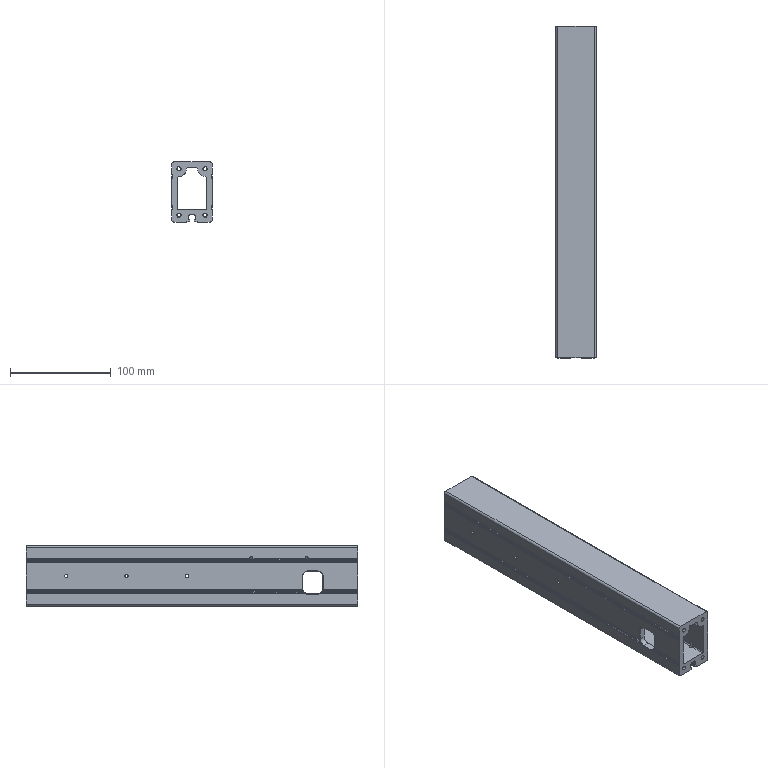Part | STEP file | 1 solid | 248 faces | box 40 x 330 x 60 mm | volume 402728 mm3 | cylinder 152 | plane 58 | cone 38 | commonest cylinder face diameters 4.2 x32 1 x30 3.3 x20 4 x16 1.3 x14 0.6 x10